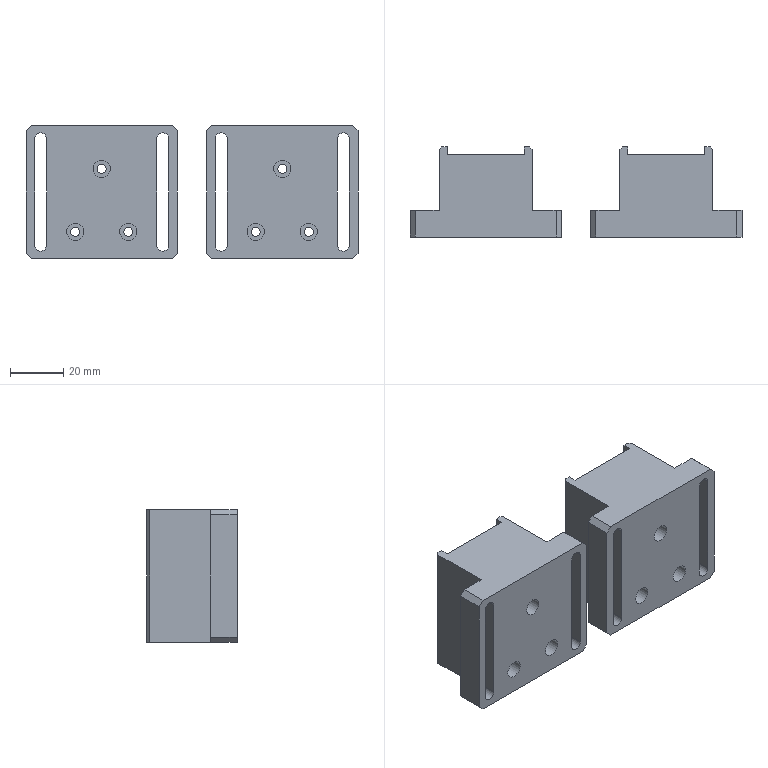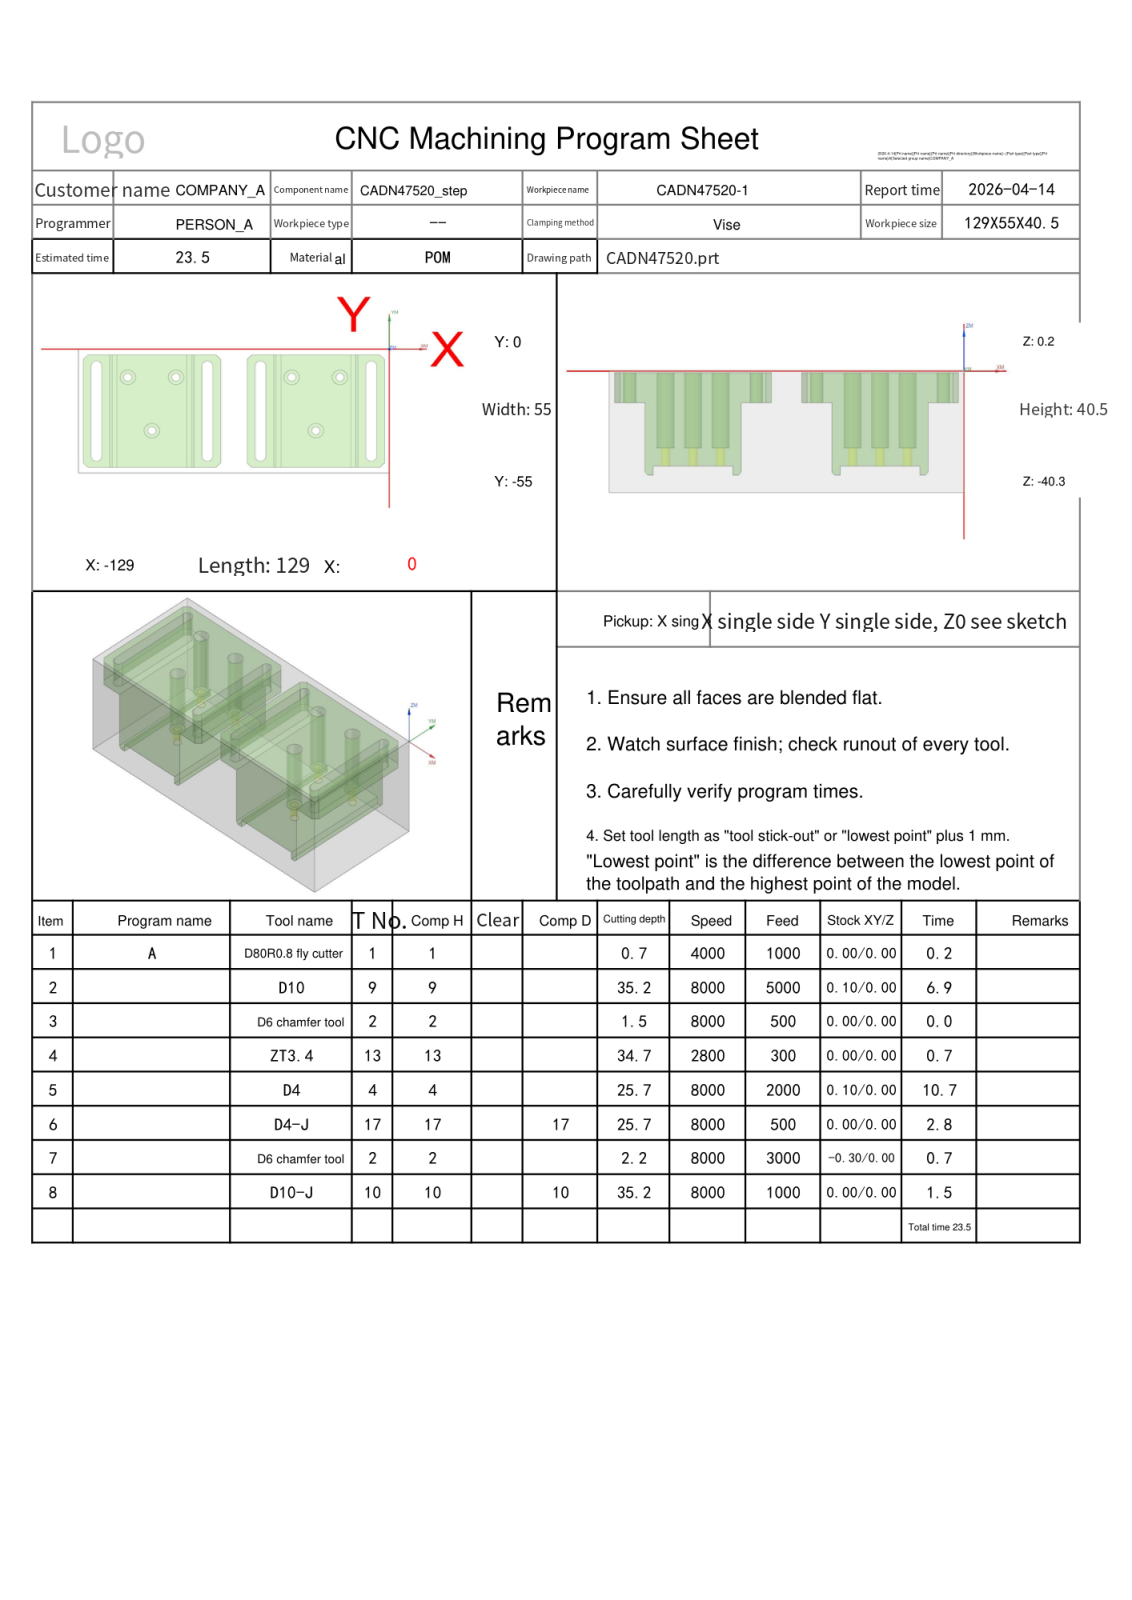NC program | NX | posted by the shop | part box 125 x 34 x 50 mm
Lines 2329 to 2380 of 5259:
N3 T02 M06
(D6 chamfer tool  D=6. R=0. H=02 ce=0.00 di=0.00)
G00 G90 G54 X-98.5 Y-36.2 M03 S8000
G43 H02 Z19.5
M08
G98 G81 X-98.5 Y-36.2 Z-1.3 R.5 F500.
X-108.5 Y-12.5
X-88.5
X-40.5
X-20.5
X-30.5 Y-36.2
X-121.5 Y-7.5
Y-47.5
X-75.5
Y-7.5
X-53.5
Y-47.5
X-7.5 Y-7.5
Y-47.5
G80
G00 Z19.5
G91 G28 Z0.0
M05
M09
G91 G28 Z0.0
M01
N4 T13 M06
(ZT3.4 D=3.4 DR_a=118 H=13)
G00 G90 G54 X-98.5 Y-36.2 M03 S2800
G43 H13 Z19.5
M08
G98 G83 X-98.5 Y-36.2 Z-34.521 R.5 F300. Q2.
X-108.5 Y-12.5
X-88.5
X-40.5
X-20.5
X-30.5 Y-36.2
G98 G83 X-121.5 Y-7.5 Z-13.521 R.5 Q2.
Y-47.5
X-75.5 Y-7.5
Y-47.5
X-53.5 Y-7.5
Y-47.5
X-7.5 Y-7.5
Y-47.5
G80
G00 Z19.5
G91 G28 Z0.0
M05
M09
G91 G28 Z0.0
M01